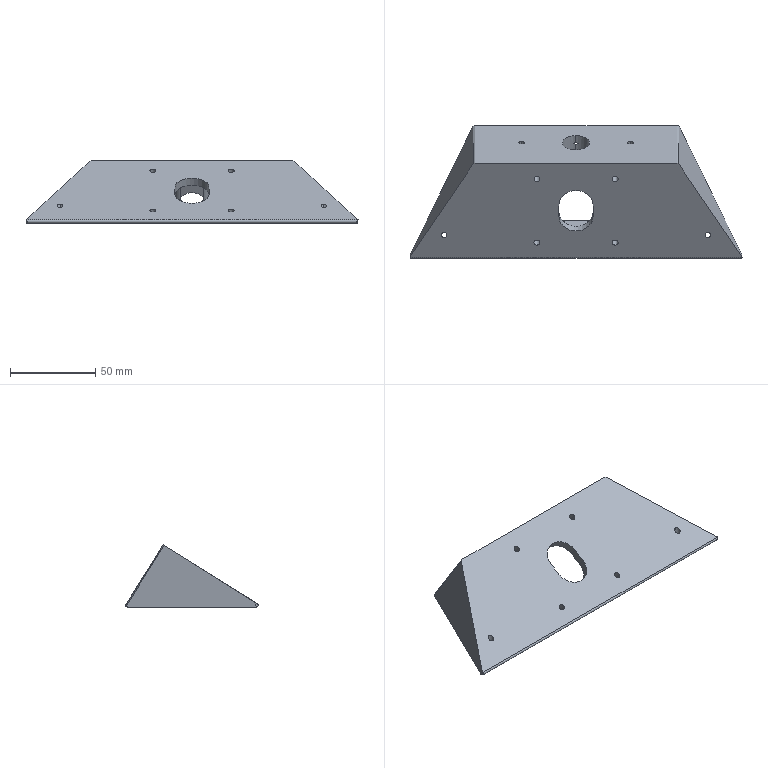Part | 1 solid | 79 faces | volume 92002 mm3 | cylinder 48 | plane 31 | commonest cylinder face diameters 3.3 x16 6 x10 3.5 x8 10 x6 2 x4 16 x2